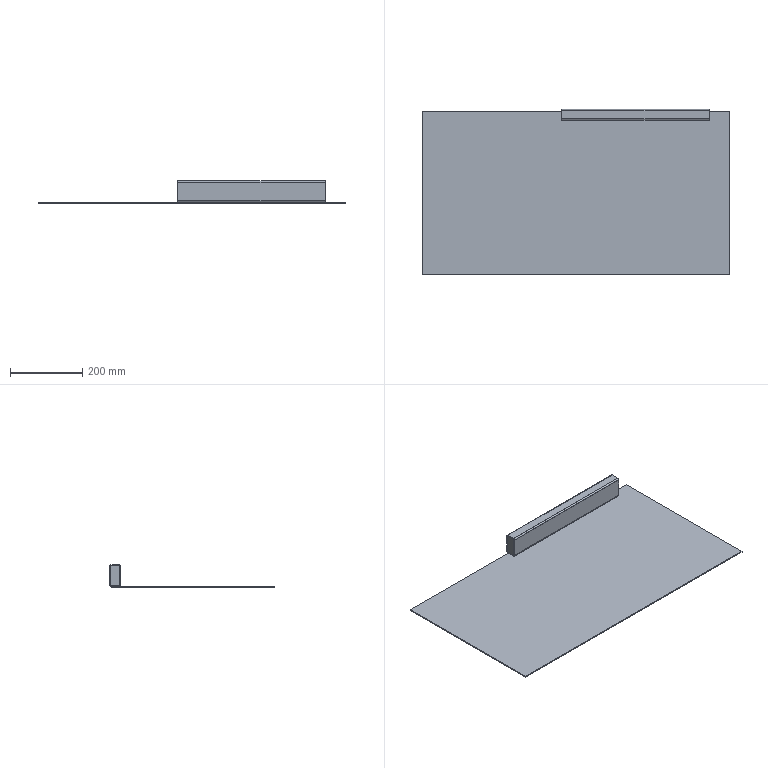Part | SolidWorks | features EndCap 1, Extrusion 1, WeldMemberFeat 1, WeldmentFeature 1 | 3 solids | 34 faces | box 850 x 458 x 63 mm | volume 1296033 mm3 | plane 22 | cylinder 12 | commonest cylinder face diameters 4 x8 8 x4
STEP:
#1=CARTESIAN_POINT('',(425.,-226.5,-1.5));
#2=VERTEX_POINT('',#1);
#3=CARTESIAN_POINT('',(425.,226.5,-1.5));
#4=VERTEX_POINT('',#3);
#5=CARTESIAN_POINT('',(425.,226.5,-1.5));
#6=DIRECTION('',(0.,1.,0.));
#7=VECTOR('',#6,1000.);
#8=LINE('',#5,#7);
#9=EDGE_CURVE('',#2,#4,#8,.T.);
#10=ORIENTED_EDGE('',*,*,#9,.T.);
#11=CARTESIAN_POINT('',(425.,226.5,1.5));
#12=VERTEX_POINT('',#11);
#13=CARTESIAN_POINT('',(425.,226.5,1.5));
#14=DIRECTION('',(0.,0.,-1.));
#15=VECTOR('',#14,1000.);
#16=LINE('',#13,#15);
#17=EDGE_CURVE('',#12,#4,#16,.T.);
#18=ORIENTED_EDGE('',*,*,#17,.F.);
#19=CARTESIAN_POINT('',(425.,-226.5,1.5));
#20=VERTEX_POINT('',#19);
#21=CARTESIAN_POINT('',(425.,226.5,1.5));
#22=DIRECTION('',(0.,1.,0.));
#23=VECTOR('',#22,1000.);
#24=LINE('',#21,#23);
#25=EDGE_CURVE('',#20,#12,#24,.T.);
#26=ORIENTED_EDGE('',*,*,#25,.F.);
#27=CARTESIAN_POINT('',(425.,-226.5,1.5));
#28=DIRECTION('',(0.,0.,-1.));
#29=VECTOR('',#28,1000.);
#30=LINE('',#27,#29);
#31=EDGE_CURVE('',#20,#2,#30,.T.);
#32=ORIENTED_EDGE('',*,*,#31,.T.);
#33=EDGE_LOOP('',(#10,#18,#26,#32));
#34=FACE_OUTER_BOUND('',#33,.T.);
#35=CARTESIAN_POINT('',(425.,226.5,1.5));
#36=DIRECTION('',(-1.,0.,0.));
#37=DIRECTION('',(0.,0.,1.));
#38=AXIS2_PLACEMENT_3D('',#35,#36,#37);
#39=PLANE('',#38);
#40=ADVANCED_FACE('',(#34),#39,.F.);
#41=CARTESIAN_POINT('',(-425.,226.5,-1.5));
#42=VERTEX_POINT('',#41);
#43=CARTESIAN_POINT('',(-425.,226.5,-1.5));
#44=DIRECTION('',(-1.,0.,0.));
#45=VECTOR('',#44,1000.);
#46=LINE('',#43,#45);
#47=EDGE_CURVE('',#4,#42,#46,.T.);
#48=ORIENTED_EDGE('',*,*,#47,.T.);
#49=CARTESIAN_POINT('',(-425.,226.5,1.5));
#50=VERTEX_POINT('',#49);
#51=CARTESIAN_POINT('',(-425.,226.5,1.5));
#52=DIRECTION('',(0.,0.,-1.));
#53=VECTOR('',#52,1000.);
#54=LINE('',#51,#53);
#55=EDGE_CURVE('',#50,#42,#54,.T.);
#56=ORIENTED_EDGE('',*,*,#55,.F.);
#57=CARTESIAN_POINT('',(-425.,226.5,1.5));
#58=DIRECTION('',(-1.,0.,0.));
#59=VECTOR('',#58,1000.);
#60=LINE('',#57,#59);
#61=EDGE_CURVE('',#12,#50,#60,.T.);
#62=ORIENTED_EDGE('',*,*,#61,.F.);
#63=ORIENTED_EDGE('',*,*,#17,.T.);
#64=EDGE_LOOP('',(#48,#56,#62,#63));
#65=FACE_OUTER_BOUND('',#64,.T.);
#66=CARTESIAN_POINT('',(-425.,226.5,1.5));
#67=DIRECTION('',(0.,-1.,0.));
#68=DIRECTION('',(0.,0.,-1.));
#69=AXIS2_PLACEMENT_3D('',#66,#67,#68);
#70=PLANE('',#69);
#71=ADVANCED_FACE('',(#65),#70,.F.);
#72=CARTESIAN_POINT('',(-425.,-226.5,-1.5));
#73=VERTEX_POINT('',#72);
#74=CARTESIAN_POINT('',(-425.,226.5,-1.5));
#75=DIRECTION('',(0.,-1.,0.));
#76=VECTOR('',#75,1000.);
#77=LINE('',#74,#76);
#78=EDGE_CURVE('',#42,#73,#77,.T.);
#79=ORIENTED_EDGE('',*,*,#78,.T.);
#80=CARTESIAN_POINT('',(-425.,-226.5,1.5));
#81=VERTEX_POINT('',#80);
#82=CARTESIAN_POINT('',(-425.,-226.5,1.5));
#83=DIRECTION('',(0.,0.,-1.));
#84=VECTOR('',#83,1000.);
#85=LINE('',#82,#84);
#86=EDGE_CURVE('',#81,#73,#85,.T.);
#87=ORIENTED_EDGE('',*,*,#86,.F.);
#88=CARTESIAN_POINT('',(-425.,226.5,1.5));
#89=DIRECTION('',(0.,-1.,0.));
#90=VECTOR('',#89,1000.);
#91=LINE('',#88,#90);
#92=EDGE_CURVE('',#50,#81,#91,.T.);
#93=ORIENTED_EDGE('',*,*,#92,.F.);
#94=ORIENTED_EDGE('',*,*,#55,.T.);
#95=EDGE_LOOP('',(#79,#87,#93,#94));
#96=FACE_OUTER_BOUND('',#95,.T.);
#97=CARTESIAN_POINT('',(-425.,226.5,1.5));
#98=DIRECTION('',(1.,0.,0.));
#99=DIRECTION('',(0.,0.,-1.));
#100=AXIS2_PLACEMENT_3D('',#97,#98,#99);
#101=PLANE('',#100);
#102=ADVANCED_FACE('',(#96),#101,.F.);
#103=CARTESIAN_POINT('',(-425.,-226.5,-1.5));
#104=DIRECTION('',(1.,0.,0.));
#105=VECTOR('',#104,1000.);
#106=LINE('',#103,#105);
#107=EDGE_CURVE('',#73,#2,#106,.T.);
#108=ORIENTED_EDGE('',*,*,#107,.T.);
#109=ORIENTED_EDGE('',*,*,#31,.F.);
#110=CARTESIAN_POINT('',(-425.,-226.5,1.5));
#111=DIRECTION('',(1.,0.,0.));
#112=VECTOR('',#111,1000.);
#113=LINE('',#110,#112);
#114=EDGE_CURVE('',#81,#20,#113,.T.);
#115=ORIENTED_EDGE('',*,*,#114,.F.);
#116=ORIENTED_EDGE('',*,*,#86,.T.);
#117=EDGE_LOOP('',(#108,#109,#115,#116));
#118=FACE_OUTER_BOUND('',#117,.T.);
#119=CARTESIAN_POINT('',(-425.,-226.5,1.5));
#120=DIRECTION('',(0.,1.,0.));
#121=DIRECTION('',(0.,0.,1.));
#122=AXIS2_PLACEMENT_3D('',#119,#120,#121);
#123=PLANE('',#122);
#124=ADVANCED_FACE('',(#118),#123,.F.);
#125=ORIENTED_EDGE('',*,*,#25,.T.);
#126=ORIENTED_EDGE('',*,*,#61,.T.);
#127=ORIENTED_EDGE('',*,*,#92,.T.);
#128=ORIENTED_EDGE('',*,*,#114,.T.);
#129=EDGE_LOOP('',(#125,#126,#127,#128));
#130=FACE_OUTER_BOUND('',#129,.T.);
#131=CARTESIAN_POINT('',(0.,0.,1.5));
#132=DIRECTION('',(0.,0.,1.));
#133=DIRECTION('',(1.,0.,0.));
#134=AXIS2_PLACEMENT_3D('',#131,#132,#133);
#135=PLANE('',#134);
#136=ADVANCED_FACE('',(#130),#135,.T.);
#137=ORIENTED_EDGE('',*,*,#9,.F.);
#138=ORIENTED_EDGE('',*,*,#107,.F.);
#139=ORIENTED_EDGE('',*,*,#78,.F.);
#140=ORIENTED_EDGE('',*,*,#47,.F.);
#141=EDGE_LOOP('',(#137,#138,#139,#140));
#142=FACE_OUTER_BOUND('',#141,.T.);
#143=CARTESIAN_POINT('',(0.,0.,-1.5));
#144=DIRECTION('',(0.,0.,1.));
#145=DIRECTION('',(1.,0.,0.));
#146=AXIS2_PLACEMENT_3D('',#143,#144,#145);
#147=PLANE('',#146);
#148=ADVANCED_FACE('',(#142),#147,.F.);
#149=CLOSED_SHELL('',(#40,#71,#102,#124,#136,#148));
#150=MANIFOLD_SOLID_BREP('',#149);
#151=CARTESIAN_POINT('',(370.,201.5,57.5));
#152=VERTEX_POINT('',#151);
#153=CARTESIAN_POINT('',(370.,205.5,61.5));
#154=VERTEX_POINT('',#153);
#155=CARTESIAN_POINT('',(370.,205.5,57.5));
#156=DIRECTION('',(-1.,0.,0.));
#157=DIRECTION('',(0.,-1.,0.));
#158=AXIS2_PLACEMENT_3D('',#155,#156,#157);
#159=CIRCLE('',#158,4.);
#160=EDGE_CURVE('',#152,#154,#159,.T.);
#161=ORIENTED_EDGE('',*,*,#160,.T.);
#162=CARTESIAN_POINT('',(-40.,205.5,61.5));
#163=VERTEX_POINT('',#162);
#164=CARTESIAN_POINT('',(-40.,205.5,61.5));
#165=DIRECTION('',(1.,0.,0.));
#166=VECTOR('',#165,1000.);
#167=LINE('',#164,#166);
#168=EDGE_CURVE('',#163,#154,#167,.T.);
#169=ORIENTED_EDGE('',*,*,#168,.F.);
#170=CARTESIAN_POINT('',(-40.,201.5,57.5));
#171=VERTEX_POINT('',#170);
#172=CARTESIAN_POINT('',(-40.,205.5,57.5));
#173=DIRECTION('',(-1.,0.,0.));
#174=DIRECTION('',(0.,-1.,0.));
#175=AXIS2_PLACEMENT_3D('',#172,#173,#174);
#176=CIRCLE('',#175,4.);
#177=EDGE_CURVE('',#171,#163,#176,.T.);
#178=ORIENTED_EDGE('',*,*,#177,.F.);
#179=CARTESIAN_POINT('',(-40.,201.5,57.5));
#180=DIRECTION('',(1.,0.,0.));
#181=VECTOR('',#180,1000.);
#182=LINE('',#179,#181);
#183=EDGE_CURVE('',#171,#152,#182,.T.);
#184=ORIENTED_EDGE('',*,*,#183,.T.);
#185=EDGE_LOOP('',(#161,#169,#178,#184));
#186=FACE_OUTER_BOUND('',#185,.T.);
#187=CARTESIAN_POINT('',(-40.,205.5,57.5));
#188=DIRECTION('',(1.,0.,0.));
#189=DIRECTION('',(0.,1.,0.));
#190=AXIS2_PLACEMENT_3D('',#187,#188,#189);
#191=CYLINDRICAL_SURFACE('',#190,4.);
#192=ADVANCED_FACE('',(#186),#191,.T.);
#193=CARTESIAN_POINT('',(370.,227.5,61.5));
#194=VERTEX_POINT('',#193);
#195=CARTESIAN_POINT('',(370.,205.5,61.5));
#196=DIRECTION('',(0.,1.,0.));
#197=VECTOR('',#196,1000.);
#198=LINE('',#195,#197);
#199=EDGE_CURVE('',#154,#194,#198,.T.);
#200=ORIENTED_EDGE('',*,*,#199,.T.);
#201=CARTESIAN_POINT('',(-40.,227.5,61.5));
#202=VERTEX_POINT('',#201);
#203=CARTESIAN_POINT('',(-40.,227.5,61.5));
#204=DIRECTION('',(1.,0.,0.));
#205=VECTOR('',#204,1000.);
#206=LINE('',#203,#205);
#207=EDGE_CURVE('',#202,#194,#206,.T.);
#208=ORIENTED_EDGE('',*,*,#207,.F.);
#209=CARTESIAN_POINT('',(-40.,205.5,61.5));
#210=DIRECTION('',(0.,1.,0.));
#211=VECTOR('',#210,1000.);
#212=LINE('',#209,#211);
#213=EDGE_CURVE('',#163,#202,#212,.T.);
#214=ORIENTED_EDGE('',*,*,#213,.F.);
#215=ORIENTED_EDGE('',*,*,#168,.T.);
#216=EDGE_LOOP('',(#200,#208,#214,#215));
#217=FACE_OUTER_BOUND('',#216,.T.);
#218=CARTESIAN_POINT('',(-40.,205.5,61.5));
#219=DIRECTION('',(0.,0.,-1.));
#220=DIRECTION('',(-1.,0.,0.));
#221=AXIS2_PLACEMENT_3D('',#218,#219,#220);
#222=PLANE('',#221);
#223=ADVANCED_FACE('',(#217),#222,.F.);
#224=CARTESIAN_POINT('',(370.,231.5,57.5));
#225=VERTEX_POINT('',#224);
#226=CARTESIAN_POINT('',(370.,227.5,57.5));
#227=DIRECTION('',(-1.,0.,0.));
#228=DIRECTION('',(0.,-1.,0.));
#229=AXIS2_PLACEMENT_3D('',#226,#227,#228);
#230=CIRCLE('',#229,4.);
#231=EDGE_CURVE('',#194,#225,#230,.T.);
#232=ORIENTED_EDGE('',*,*,#231,.T.);
#233=CARTESIAN_POINT('',(-40.,231.5,57.5));
#234=VERTEX_POINT('',#233);
#235=CARTESIAN_POINT('',(-40.,231.5,57.5));
#236=DIRECTION('',(1.,0.,0.));
#237=VECTOR('',#236,1000.);
#238=LINE('',#235,#237);
#239=EDGE_CURVE('',#234,#225,#238,.T.);
#240=ORIENTED_EDGE('',*,*,#239,.F.);
#241=CARTESIAN_POINT('',(-40.,227.5,57.5));
#242=DIRECTION('',(-1.,0.,0.));
#243=DIRECTION('',(0.,-1.,0.));
#244=AXIS2_PLACEMENT_3D('',#241,#242,#243);
#245=CIRCLE('',#244,4.);
#246=EDGE_CURVE('',#202,#234,#245,.T.);
#247=ORIENTED_EDGE('',*,*,#246,.F.);
#248=ORIENTED_EDGE('',*,*,#207,.T.);
#249=EDGE_LOOP('',(#232,#240,#247,#248));
#250=FACE_OUTER_BOUND('',#249,.T.);
#251=CARTESIAN_POINT('',(-40.,227.5,57.5));
#252=DIRECTION('',(1.,0.,0.));
#253=DIRECTION('',(0.,1.,0.));
#254=AXIS2_PLACEMENT_3D('',#251,#252,#253);
#255=CYLINDRICAL_SURFACE('',#254,4.);
#256=ADVANCED_FACE('',(#250),#255,.T.);
#257=CARTESIAN_POINT('',(370.,231.5,5.5));
#258=VERTEX_POINT('',#257);
#259=CARTESIAN_POINT('',(370.,231.5,5.5));
#260=DIRECTION('',(0.,0.,-1.));
#261=VECTOR('',#260,1000.);
#262=LINE('',#259,#261);
#263=EDGE_CURVE('',#225,#258,#262,.T.);
#264=ORIENTED_EDGE('',*,*,#263,.T.);
#265=CARTESIAN_POINT('',(-40.,231.5,5.5));
#266=VERTEX_POINT('',#265);
#267=CARTESIAN_POINT('',(-40.,231.5,5.5));
#268=DIRECTION('',(1.,0.,0.));
#269=VECTOR('',#268,1000.);
#270=LINE('',#267,#269);
#271=EDGE_CURVE('',#266,#258,#270,.T.);
#272=ORIENTED_EDGE('',*,*,#271,.F.);
#273=CARTESIAN_POINT('',(-40.,231.5,5.5));
#274=DIRECTION('',(0.,0.,-1.));
#275=VECTOR('',#274,1000.);
#276=LINE('',#273,#275);
#277=EDGE_CURVE('',#234,#266,#276,.T.);
#278=ORIENTED_EDGE('',*,*,#277,.F.);
#279=ORIENTED_EDGE('',*,*,#239,.T.);
#280=EDGE_LOOP('',(#264,#272,#278,#279));
#281=FACE_OUTER_BOUND('',#280,.T.);
#282=CARTESIAN_POINT('',(-40.,231.5,5.5));
#283=DIRECTION('',(0.,-1.,0.));
#284=DIRECTION('',(1.,0.,0.));
#285=AXIS2_PLACEMENT_3D('',#282,#283,#284);
#286=PLANE('',#285);
#287=ADVANCED_FACE('',(#281),#286,.F.);
#288=CARTESIAN_POINT('',(370.,227.5,1.5));
#289=VERTEX_POINT('',#288);
#290=CARTESIAN_POINT('',(370.,227.5,5.5));
#291=DIRECTION('',(-1.,0.,0.));
#292=DIRECTION('',(0.,-1.,0.));
#293=AXIS2_PLACEMENT_3D('',#290,#291,#292);
#294=CIRCLE('',#293,4.);
#295=EDGE_CURVE('',#258,#289,#294,.T.);
#296=ORIENTED_EDGE('',*,*,#295,.T.);
#297=CARTESIAN_POINT('',(-40.,227.5,1.5));
#298=VERTEX_POINT('',#297);
#299=CARTESIAN_POINT('',(-40.,227.5,1.5));
#300=DIRECTION('',(1.,0.,0.));
#301=VECTOR('',#300,1000.);
#302=LINE('',#299,#301);
#303=EDGE_CURVE('',#298,#289,#302,.T.);
#304=ORIENTED_EDGE('',*,*,#303,.F.);
#305=CARTESIAN_POINT('',(-40.,227.5,5.5));
#306=DIRECTION('',(-1.,0.,0.));
#307=DIRECTION('',(0.,-1.,0.));
#308=AXIS2_PLACEMENT_3D('',#305,#306,#307);
#309=CIRCLE('',#308,4.);
#310=EDGE_CURVE('',#266,#298,#309,.T.);
#311=ORIENTED_EDGE('',*,*,#310,.F.);
#312=ORIENTED_EDGE('',*,*,#271,.T.);
#313=EDGE_LOOP('',(#296,#304,#311,#312));
#314=FACE_OUTER_BOUND('',#313,.T.);
#315=CARTESIAN_POINT('',(-40.,227.5,5.5));
#316=DIRECTION('',(1.,0.,0.));
#317=DIRECTION('',(0.,1.,0.));
#318=AXIS2_PLACEMENT_3D('',#315,#316,#317);
#319=CYLINDRICAL_SURFACE('',#318,4.);
#320=ADVANCED_FACE('',(#314),#319,.T.);
#321=CARTESIAN_POINT('',(370.,205.5,1.5));
#322=VERTEX_POINT('',#321);
#323=CARTESIAN_POINT('',(370.,227.5,1.5));
#324=DIRECTION('',(0.,-1.,0.));
#325=VECTOR('',#324,1000.);
#326=LINE('',#323,#325);
#327=EDGE_CURVE('',#289,#322,#326,.T.);
#328=ORIENTED_EDGE('',*,*,#327,.T.);
#329=CARTESIAN_POINT('',(-40.,205.5,1.5));
#330=VERTEX_POINT('',#329);
#331=CARTESIAN_POINT('',(-40.,205.5,1.5));
#332=DIRECTION('',(1.,0.,0.));
#333=VECTOR('',#332,1000.);
#334=LINE('',#331,#333);
#335=EDGE_CURVE('',#330,#322,#334,.T.);
#336=ORIENTED_EDGE('',*,*,#335,.F.);
#337=CARTESIAN_POINT('',(-40.,227.5,1.5));
#338=DIRECTION('',(0.,-1.,0.));
#339=VECTOR('',#338,1000.);
#340=LINE('',#337,#339);
#341=EDGE_CURVE('',#298,#330,#340,.T.);
#342=ORIENTED_EDGE('',*,*,#341,.F.);
#343=ORIENTED_EDGE('',*,*,#303,.T.);
#344=EDGE_LOOP('',(#328,#336,#342,#343));
#345=FACE_OUTER_BOUND('',#344,.T.);
#346=CARTESIAN_POINT('',(-40.,227.5,1.5));
#347=DIRECTION('',(0.,0.,1.));
#348=DIRECTION('',(1.,0.,0.));
#349=AXIS2_PLACEMENT_3D('',#346,#347,#348);
#350=PLANE('',#349);
#351=ADVANCED_FACE('',(#345),#350,.F.);
#352=CARTESIAN_POINT('',(370.,201.5,5.5));
#353=VERTEX_POINT('',#352);
#354=CARTESIAN_POINT('',(370.,205.5,5.5));
#355=DIRECTION('',(-1.,0.,0.));
#356=DIRECTION('',(0.,-1.,0.));
#357=AXIS2_PLACEMENT_3D('',#354,#355,#356);
#358=CIRCLE('',#357,4.);
#359=EDGE_CURVE('',#322,#353,#358,.T.);
#360=ORIENTED_EDGE('',*,*,#359,.T.);
#361=CARTESIAN_POINT('',(-40.,201.5,5.5));
#362=VERTEX_POINT('',#361);
#363=CARTESIAN_POINT('',(-40.,201.5,5.5));
#364=DIRECTION('',(1.,0.,0.));
#365=VECTOR('',#364,1000.);
#366=LINE('',#363,#365);
#367=EDGE_CURVE('',#362,#353,#366,.T.);
#368=ORIENTED_EDGE('',*,*,#367,.F.);
#369=CARTESIAN_POINT('',(-40.,205.5,5.5));
#370=DIRECTION('',(-1.,0.,0.));
#371=DIRECTION('',(0.,-1.,0.));
#372=AXIS2_PLACEMENT_3D('',#369,#370,#371);
#373=CIRCLE('',#372,4.);
#374=EDGE_CURVE('',#330,#362,#373,.T.);
#375=ORIENTED_EDGE('',*,*,#374,.F.);
#376=ORIENTED_EDGE('',*,*,#335,.T.);
#377=EDGE_LOOP('',(#360,#368,#375,#376));
#378=FACE_OUTER_BOUND('',#377,.T.);
#379=CARTESIAN_POINT('',(-40.,205.5,5.5));
#380=DIRECTION('',(1.,0.,0.));
#381=DIRECTION('',(0.,1.,0.));
#382=AXIS2_PLACEMENT_3D('',#379,#380,#381);
#383=CYLINDRICAL_SURFACE('',#382,4.);
#384=ADVANCED_FACE('',(#378),#383,.T.);
#385=CARTESIAN_POINT('',(370.,227.5,59.5));
#386=VERTEX_POINT('',#385);
#387=CARTESIAN_POINT('',(370.,229.5,57.5));
#388=VERTEX_POINT('',#387);
#389=CARTESIAN_POINT('',(370.,227.5,57.5));
#390=DIRECTION('',(-1.,0.,0.));
#391=DIRECTION('',(0.,-1.,0.));
#392=AXIS2_PLACEMENT_3D('',#389,#390,#391);
#393=CIRCLE('',#392,2.);
#394=EDGE_CURVE('',#386,#388,#393,.T.);
#395=ORIENTED_EDGE('',*,*,#394,.F.);
#396=CARTESIAN_POINT('',(-40.,227.5,59.5));
#397=VERTEX_POINT('',#396);
#398=CARTESIAN_POINT('',(-40.,227.5,59.5));
#399=DIRECTION('',(1.,0.,0.));
#400=VECTOR('',#399,1000.);
#401=LINE('',#398,#400);
#402=EDGE_CURVE('',#397,#386,#401,.T.);
#403=ORIENTED_EDGE('',*,*,#402,.F.);
#404=CARTESIAN_POINT('',(-40.,229.5,57.5));
#405=VERTEX_POINT('',#404);
#406=CARTESIAN_POINT('',(-40.,227.5,57.5));
#407=DIRECTION('',(-1.,0.,0.));
#408=DIRECTION('',(0.,-1.,0.));
#409=AXIS2_PLACEMENT_3D('',#406,#407,#408);
#410=CIRCLE('',#409,2.);
#411=EDGE_CURVE('',#397,#405,#410,.T.);
#412=ORIENTED_EDGE('',*,*,#411,.T.);
#413=CARTESIAN_POINT('',(-40.,229.5,57.5));
#414=DIRECTION('',(1.,0.,0.));
#415=VECTOR('',#414,1000.);
#416=LINE('',#413,#415);
#417=EDGE_CURVE('',#405,#388,#416,.T.);
#418=ORIENTED_EDGE('',*,*,#417,.T.);
#419=EDGE_LOOP('',(#395,#403,#412,#418));
#420=FACE_OUTER_BOUND('',#419,.T.);
#421=CARTESIAN_POINT('',(-40.,227.5,57.5));
#422=DIRECTION('',(1.,0.,0.));
#423=DIRECTION('',(0.,1.,0.));
#424=AXIS2_PLACEMENT_3D('',#421,#422,#423);
#425=CYLINDRICAL_SURFACE('',#424,2.);
#426=ADVANCED_FACE('',(#420),#425,.F.);
#427=CARTESIAN_POINT('',(370.,205.5,59.5));
#428=VERTEX_POINT('',#427);
#429=CARTESIAN_POINT('',(370.,205.5,59.5));
#430=DIRECTION('',(0.,1.,0.));
#431=VECTOR('',#430,1000.);
#432=LINE('',#429,#431);
#433=EDGE_CURVE('',#428,#386,#432,.T.);
#434=ORIENTED_EDGE('',*,*,#433,.F.);
#435=CARTESIAN_POINT('',(-40.,205.5,59.5));
#436=VERTEX_POINT('',#435);
#437=CARTESIAN_POINT('',(-40.,205.5,59.5));
#438=DIRECTION('',(1.,0.,0.));
#439=VECTOR('',#438,1000.);
#440=LINE('',#437,#439);
#441=EDGE_CURVE('',#436,#428,#440,.T.);
#442=ORIENTED_EDGE('',*,*,#441,.F.);
#443=CARTESIAN_POINT('',(-40.,205.5,59.5));
#444=DIRECTION('',(0.,1.,0.));
#445=VECTOR('',#444,1000.);
#446=LINE('',#443,#445);
#447=EDGE_CURVE('',#436,#397,#446,.T.);
#448=ORIENTED_EDGE('',*,*,#447,.T.);
#449=ORIENTED_EDGE('',*,*,#402,.T.);
#450=EDGE_LOOP('',(#434,#442,#448,#449));
#451=FACE_OUTER_BOUND('',#450,.T.);
#452=CARTESIAN_POINT('',(-40.,205.5,59.5));
#453=DIRECTION('',(0.,0.,-1.));
#454=DIRECTION('',(-1.,0.,0.));
#455=AXIS2_PLACEMENT_3D('',#452,#453,#454);
#456=PLANE('',#455);
#457=ADVANCED_FACE('',(#451),#456,.T.);
#458=CARTESIAN_POINT('',(370.,203.5,57.5));
#459=VERTEX_POINT('',#458);
#460=CARTESIAN_POINT('',(370.,205.5,57.5));
#461=DIRECTION('',(-1.,0.,0.));
#462=DIRECTION('',(0.,-1.,0.));
#463=AXIS2_PLACEMENT_3D('',#460,#461,#462);
#464=CIRCLE('',#463,2.);
#465=EDGE_CURVE('',#459,#428,#464,.T.);
#466=ORIENTED_EDGE('',*,*,#465,.F.);
#467=CARTESIAN_POINT('',(-40.,203.5,57.5));
#468=VERTEX_POINT('',#467);
#469=CARTESIAN_POINT('',(-40.,203.5,57.5));
#470=DIRECTION('',(1.,0.,0.));
#471=VECTOR('',#470,1000.);
#472=LINE('',#469,#471);
#473=EDGE_CURVE('',#468,#459,#472,.T.);
#474=ORIENTED_EDGE('',*,*,#473,.F.);
#475=CARTESIAN_POINT('',(-40.,205.5,57.5));
#476=DIRECTION('',(-1.,0.,0.));
#477=DIRECTION('',(0.,-1.,0.));
#478=AXIS2_PLACEMENT_3D('',#475,#476,#477);
#479=CIRCLE('',#478,2.);
#480=EDGE_CURVE('',#468,#436,#479,.T.);
#481=ORIENTED_EDGE('',*,*,#480,.T.);
#482=ORIENTED_EDGE('',*,*,#441,.T.);
#483=EDGE_LOOP('',(#466,#474,#481,#482));
#484=FACE_OUTER_BOUND('',#483,.T.);
#485=CARTESIAN_POINT('',(-40.,205.5,57.5));
#486=DIRECTION('',(1.,0.,0.));
#487=DIRECTION('',(0.,1.,0.));
#488=AXIS2_PLACEMENT_3D('',#485,#486,#487);
#489=CYLINDRICAL_SURFACE('',#488,2.);
#490=ADVANCED_FACE('',(#484),#489,.F.);
#491=CARTESIAN_POINT('',(370.,203.5,5.5));
#492=VERTEX_POINT('',#491);
#493=CARTESIAN_POINT('',(370.,203.5,57.5));
#494=DIRECTION('',(0.,0.,1.));
#495=VECTOR('',#494,1000.);
#496=LINE('',#493,#495);
#497=EDGE_CURVE('',#492,#459,#496,.T.);
#498=ORIENTED_EDGE('',*,*,#497,.F.);
#499=CARTESIAN_POINT('',(-40.,203.5,5.5));
#500=VERTEX_POINT('',#499);
#501=CARTESIAN_POINT('',(-40.,203.5,5.5));
#502=DIRECTION('',(1.,0.,0.));
#503=VECTOR('',#502,1000.);
#504=LINE('',#501,#503);
#505=EDGE_CURVE('',#500,#492,#504,.T.);
#506=ORIENTED_EDGE('',*,*,#505,.F.);
#507=CARTESIAN_POINT('',(-40.,203.5,57.5));
#508=DIRECTION('',(0.,0.,1.));
#509=VECTOR('',#508,1000.);
#510=LINE('',#507,#509);
#511=EDGE_CURVE('',#500,#468,#510,.T.);
#512=ORIENTED_EDGE('',*,*,#511,.T.);
#513=ORIENTED_EDGE('',*,*,#473,.T.);
#514=EDGE_LOOP('',(#498,#506,#512,#513));
#515=FACE_OUTER_BOUND('',#514,.T.);
#516=CARTESIAN_POINT('',(-40.,203.5,57.5));
#517=DIRECTION('',(0.,1.,0.));
#518=DIRECTION('',(-1.,0.,0.));
#519=AXIS2_PLACEMENT_3D('',#516,#517,#518);
#520=PLANE('',#519);
#521=ADVANCED_FACE('',(#515),#520,.T.);
#522=CARTESIAN_POINT('',(370.,205.5,3.5));
#523=VERTEX_POINT('',#522);
#524=CARTESIAN_POINT('',(370.,205.5,5.5));
#525=DIRECTION('',(-1.,0.,0.));
#526=DIRECTION('',(0.,-1.,0.));
#527=AXIS2_PLACEMENT_3D('',#524,#525,#526);
#528=CIRCLE('',#527,2.);
#529=EDGE_CURVE('',#523,#492,#528,.T.);
#530=ORIENTED_EDGE('',*,*,#529,.F.);
#531=CARTESIAN_POINT('',(-40.,205.5,3.5));
#532=VERTEX_POINT('',#531);
#533=CARTESIAN_POINT('',(-40.,205.5,3.5));
#534=DIRECTION('',(1.,0.,0.));
#535=VECTOR('',#534,1000.);
#536=LINE('',#533,#535);
#537=EDGE_CURVE('',#532,#523,#536,.T.);
#538=ORIENTED_EDGE('',*,*,#537,.F.);
#539=CARTESIAN_POINT('',(-40.,205.5,5.5));
#540=DIRECTION('',(-1.,0.,0.));
#541=DIRECTION('',(0.,-1.,0.));
#542=AXIS2_PLACEMENT_3D('',#539,#540,#541);
#543=CIRCLE('',#542,2.);
#544=EDGE_CURVE('',#532,#500,#543,.T.);
#545=ORIENTED_EDGE('',*,*,#544,.T.);
#546=ORIENTED_EDGE('',*,*,#505,.T.);
#547=EDGE_LOOP('',(#530,#538,#545,#546));
#548=FACE_OUTER_BOUND('',#547,.T.);
#549=CARTESIAN_POINT('',(-40.,205.5,5.5));
#550=DIRECTION('',(1.,0.,0.));
#551=DIRECTION('',(0.,1.,0.));
#552=AXIS2_PLACEMENT_3D('',#549,#550,#551);
#553=CYLINDRICAL_SURFACE('',#552,2.);
#554=ADVANCED_FACE('',(#548),#553,.F.);
#555=CARTESIAN_POINT('',(370.,227.5,3.5));
#556=VERTEX_POINT('',#555);
#557=CARTESIAN_POINT('',(370.,227.5,3.5));
#558=DIRECTION('',(0.,-1.,0.));
#559=VECTOR('',#558,1000.);
#560=LINE('',#557,#559);
#561=EDGE_CURVE('',#556,#523,#560,.T.);
#562=ORIENTED_EDGE('',*,*,#561,.F.);
#563=CARTESIAN_POINT('',(-40.,227.5,3.5));
#564=VERTEX_POINT('',#563);
#565=CARTESIAN_POINT('',(-40.,227.5,3.5));
#566=DIRECTION('',(1.,0.,0.));
#567=VECTOR('',#566,1000.);
#568=LINE('',#565,#567);
#569=EDGE_CURVE('',#564,#556,#568,.T.);
#570=ORIENTED_EDGE('',*,*,#569,.F.);
#571=CARTESIAN_POINT('',(-40.,227.5,3.5));
#572=DIRECTION('',(0.,-1.,0.));
#573=VECTOR('',#572,1000.);
#574=LINE('',#571,#573);
#575=EDGE_CURVE('',#564,#532,#574,.T.);
#576=ORIENTED_EDGE('',*,*,#575,.T.);
#577=ORIENTED_EDGE('',*,*,#537,.T.);
#578=EDGE_LOOP('',(#562,#570,#576,#577));
#579=FACE_OUTER_BOUND('',#578,.T.);
#580=CARTESIAN_POINT('',(-40.,227.5,3.5));
#581=DIRECTION('',(0.,0.,1.));
#582=DIRECTION('',(1.,0.,0.));
#583=AXIS2_PLACEMENT_3D('',#580,#581,#582);
#584=PLANE('',#583);
#585=ADVANCED_FACE('',(#579),#584,.T.);
#586=CARTESIAN_POINT('',(370.,229.5,5.5));
#587=VERTEX_POINT('',#586);
#588=CARTESIAN_POINT('',(370.,227.5,5.5));
#589=DIRECTION('',(-1.,0.,0.));
#590=DIRECTION('',(0.,-1.,0.));
#591=AXIS2_PLACEMENT_3D('',#588,#589,#590);
#592=CIRCLE('',#591,2.);
#593=EDGE_CURVE('',#587,#556,#592,.T.);
#594=ORIENTED_EDGE('',*,*,#593,.F.);
#595=CARTESIAN_POINT('',(-40.,229.5,5.5));
#596=VERTEX_POINT('',#595);
#597=CARTESIAN_POINT('',(-40.,229.5,5.5));
#598=DIRECTION('',(1.,0.,0.));
#599=VECTOR('',#598,1000.);
#600=LINE('',#597,#599);
#601=EDGE_CURVE('',#596,#587,#600,.T.);
#602=ORIENTED_EDGE('',*,*,#601,.F.);
#603=CARTESIAN_POINT('',(-40.,227.5,5.5));
#604=DIRECTION('',(-1.,0.,0.));
#605=DIRECTION('',(0.,-1.,0.));
#606=AXIS2_PLACEMENT_3D('',#603,#604,#605);
#607=CIRCLE('',#606,2.);
#608=EDGE_CURVE('',#596,#564,#607,.T.);
#609=ORIENTED_EDGE('',*,*,#608,.T.);
#610=ORIENTED_EDGE('',*,*,#569,.T.);
#611=EDGE_LOOP('',(#594,#602,#609,#610));
#612=FACE_OUTER_BOUND('',#611,.T.);
#613=CARTESIAN_POINT('',(-40.,227.5,5.5));
#614=DIRECTION('',(1.,0.,0.));
#615=DIRECTION('',(0.,1.,0.));
#616=AXIS2_PLACEMENT_3D('',#613,#614,#615);
#617=CYLINDRICAL_SURFACE('',#616,2.);
#618=ADVANCED_FACE('',(#612),#617,.F.);
#619=CARTESIAN_POINT('',(370.,229.5,5.5));
#620=DIRECTION('',(0.,0.,-1.));
#621=VECTOR('',#620,1000.);
#622=LINE('',#619,#621);
#623=EDGE_CURVE('',#388,#587,#622,.T.);
#624=ORIENTED_EDGE('',*,*,#623,.F.);
#625=ORIENTED_EDGE('',*,*,#417,.F.);
#626=CARTESIAN_POINT('',(-40.,229.5,5.5));
#627=DIRECTION('',(0.,0.,-1.));
#628=VECTOR('',#627,1000.);
#629=LINE('',#626,#628);
#630=EDGE_CURVE('',#405,#596,#629,.T.);
#631=ORIENTED_EDGE('',*,*,#630,.T.);
#632=ORIENTED_EDGE('',*,*,#601,.T.);
#633=EDGE_LOOP('',(#624,#625,#631,#632));
#634=FACE_OUTER_BOUND('',#633,.T.);
#635=CARTESIAN_POINT('',(-40.,229.5,5.5));
#636=DIRECTION('',(0.,-1.,0.));
#637=DIRECTION('',(1.,0.,0.));
#638=AXIS2_PLACEMENT_3D('',#635,#636,#637);
#639=PLANE('',#638);
#640=ADVANCED_FACE('',(#634),#639,.T.);
#641=CARTESIAN_POINT('',(370.,201.5,57.5));
#642=DIRECTION('',(0.,0.,1.));
#643=VECTOR('',#642,1000.);
#644=LINE('',#641,#643);
#645=EDGE_CURVE('',#353,#152,#644,.T.);
#646=ORIENTED_EDGE('',*,*,#645,.T.);
#647=ORIENTED_EDGE('',*,*,#183,.F.);
#648=CARTESIAN_POINT('',(-40.,201.5,57.5));
#649=DIRECTION('',(0.,0.,1.));
#650=VECTOR('',#649,1000.);
#651=LINE('',#648,#650);
#652=EDGE_CURVE('',#362,#171,#651,.T.);
#653=ORIENTED_EDGE('',*,*,#652,.F.);
#654=ORIENTED_EDGE('',*,*,#367,.T.);
#655=EDGE_LOOP('',(#646,#647,#653,#654));
#656=FACE_OUTER_BOUND('',#655,.T.);
#657=CARTESIAN_POINT('',(-40.,201.5,57.5));
#658=DIRECTION('',(0.,1.,0.));
#659=DIRECTION('',(-1.,0.,0.));
#660=AXIS2_PLACEMENT_3D('',#657,#658,#659);
#661=PLANE('',#660);
#662=ADVANCED_FACE('',(#656),#661,.F.);
#663=ORIENTED_EDGE('',*,*,#411,.F.);
#664=ORIENTED_EDGE('',*,*,#447,.F.);
#665=ORIENTED_EDGE('',*,*,#480,.F.);
#666=ORIENTED_EDGE('',*,*,#511,.F.);
#667=ORIENTED_EDGE('',*,*,#544,.F.);
#668=ORIENTED_EDGE('',*,*,#575,.F.);
#669=ORIENTED_EDGE('',*,*,#608,.F.);
#670=ORIENTED_EDGE('',*,*,#630,.F.);
#671=EDGE_LOOP('',(#663,#664,#665,#666,#667,#668,#669,#670));
#672=FACE_BOUND('',#671,.T.);
#673=ORIENTED_EDGE('',*,*,#177,.T.);
#674=ORIENTED_EDGE('',*,*,#213,.T.);
#675=ORIENTED_EDGE('',*,*,#246,.T.);
#676=ORIENTED_EDGE('',*,*,#277,.T.);
#677=ORIENTED_EDGE('',*,*,#310,.T.);
#678=ORIENTED_EDGE('',*,*,#341,.T.);
#679=ORIENTED_EDGE('',*,*,#374,.T.);
#680=ORIENTED_EDGE('',*,*,#652,.T.);
#681=EDGE_LOOP('',(#673,#674,#675,#676,#677,#678,#679,#680));
#682=FACE_OUTER_BOUND('',#681,.T.);
#683=CARTESIAN_POINT('',(-40.,205.5,57.5));
#684=DIRECTION('',(-1.,0.,0.));
#685=DIRECTION('',(0.,-1.,0.));
#686=AXIS2_PLACEMENT_3D('',#683,#684,#685);
#687=PLANE('',#686);
#688=ADVANCED_FACE('',(#672,#682),#687,.T.);
#689=ORIENTED_EDGE('',*,*,#394,.T.);
#690=ORIENTED_EDGE('',*,*,#623,.T.);
#691=ORIENTED_EDGE('',*,*,#593,.T.);
#692=ORIENTED_EDGE('',*,*,#561,.T.);
#693=ORIENTED_EDGE('',*,*,#529,.T.);
#694=ORIENTED_EDGE('',*,*,#497,.T.);
#695=ORIENTED_EDGE('',*,*,#465,.T.);
#696=ORIENTED_EDGE('',*,*,#433,.T.);
#697=EDGE_LOOP('',(#689,#690,#691,#692,#693,#694,#695,#696));
#698=FACE_BOUND('',#697,.T.);
#699=ORIENTED_EDGE('',*,*,#160,.F.);
#700=ORIENTED_EDGE('',*,*,#645,.F.);
#701=ORIENTED_EDGE('',*,*,#359,.F.);
#702=ORIENTED_EDGE('',*,*,#327,.F.);
#703=ORIENTED_EDGE('',*,*,#295,.F.);
#704=ORIENTED_EDGE('',*,*,#263,.F.);
#705=ORIENTED_EDGE('',*,*,#231,.F.);
#706=ORIENTED_EDGE('',*,*,#199,.F.);
#707=EDGE_LOOP('',(#699,#700,#701,#702,#703,#704,#705,#706));
#708=FACE_OUTER_BOUND('',#707,.T.);
#709=CARTESIAN_POINT('',(370.,205.5,57.5));
#710=DIRECTION('',(-1.,0.,0.));
#711=DIRECTION('',(0.,-1.,0.));
#712=AXIS2_PLACEMENT_3D('',#709,#710,#711);
#713=PLANE('',#712);
#714=ADVANCED_FACE('',(#698,#708),#713,.F.);
#715=CLOSED_SHELL('',(#192,#223,#256,#287,#320,#351,#384,#426,#457,#490,#521,#554,#585,#618,#640,#662,#688,#714));
#716=MANIFOLD_SOLID_BREP('',#715);
#717=CARTESIAN_POINT('',(-40.,204.1,56.9));
#718=VERTEX_POINT('',#717);
#719=CARTESIAN_POINT('',(-40.,204.1,6.1));
#720=VERTEX_POINT('',#719);
#721=CARTESIAN_POINT('',(-40.,204.1,58.9));
#722=DIRECTION('',(0.,0.,-1.));
#723=VECTOR('',#722,1000.);
#724=LINE('',#721,#723);
#725=EDGE_CURVE('',#718,#720,#724,.T.);
#726=ORIENTED_EDGE('',*,*,#725,.T.);
#727=CARTESIAN_POINT('',(-37.,204.1,6.1));
#728=VERTEX_POINT('',#727);
#729=CARTESIAN_POINT('',(-37.,204.1,6.1));
#730=DIRECTION('',(-1.,0.,0.));
#731=VECTOR('',#730,1000.);
#732=LINE('',#729,#731);
#733=EDGE_CURVE('',#728,#720,#732,.T.);
#734=ORIENTED_EDGE('',*,*,#733,.F.);
#735=CARTESIAN_POINT('',(-37.,204.1,56.9));
#736=VERTEX_POINT('',#735);
#737=CARTESIAN_POINT('',(-37.,204.1,58.9));
#738=DIRECTION('',(0.,0.,-1.));
#739=VECTOR('',#738,1000.);
#740=LINE('',#737,#739);
#741=EDGE_CURVE('',#736,#728,#740,.T.);
#742=ORIENTED_EDGE('',*,*,#741,.F.);
#743=CARTESIAN_POINT('',(-37.,204.1,56.9));
#744=DIRECTION('',(-1.,0.,0.));
#745=VECTOR('',#744,1000.);
#746=LINE('',#743,#745);
#747=EDGE_CURVE('',#736,#718,#746,.T.);
#748=ORIENTED_EDGE('',*,*,#747,.T.);
#749=EDGE_LOOP('',(#726,#734,#742,#748));
#750=FACE_OUTER_BOUND('',#749,.T.);
#751=CARTESIAN_POINT('',(-37.,204.1,58.9));
#752=DIRECTION('',(0.,1.,0.));
#753=DIRECTION('',(-1.,0.,0.));
#754=AXIS2_PLACEMENT_3D('',#751,#752,#753);
#755=PLANE('',#754);
#756=ADVANCED_FACE('',(#750),#755,.F.);
#757=CARTESIAN_POINT('',(-40.,206.1,4.1));
#758=VERTEX_POINT('',#757);
#759=CARTESIAN_POINT('',(-40.,206.1,6.1));
#760=DIRECTION('',(1.,0.,0.));
#761=DIRECTION('',(0.,0.,1.));
#762=AXIS2_PLACEMENT_3D('',#759,#760,#761);
#763=CIRCLE('',#762,2.);
#764=EDGE_CURVE('',#720,#758,#763,.T.);
#765=ORIENTED_EDGE('',*,*,#764,.T.);
#766=CARTESIAN_POINT('',(-37.,206.1,4.1));
#767=VERTEX_POINT('',#766);
#768=CARTESIAN_POINT('',(-37.,206.1,4.1));
#769=DIRECTION('',(-1.,0.,0.));
#770=VECTOR('',#769,1000.);
#771=LINE('',#768,#770);
#772=EDGE_CURVE('',#767,#758,#771,.T.);
#773=ORIENTED_EDGE('',*,*,#772,.F.);
#774=CARTESIAN_POINT('',(-37.,206.1,6.1));
#775=DIRECTION('',(1.,0.,0.));
#776=DIRECTION('',(0.,0.,1.));
#777=AXIS2_PLACEMENT_3D('',#774,#775,#776);
#778=CIRCLE('',#777,2.);
#779=EDGE_CURVE('',#728,#767,#778,.T.);
#780=ORIENTED_EDGE('',*,*,#779,.F.);
#781=ORIENTED_EDGE('',*,*,#733,.T.);
#782=EDGE_LOOP('',(#765,#773,#780,#781));
#783=FACE_OUTER_BOUND('',#782,.T.);
#784=CARTESIAN_POINT('',(-37.,206.1,6.1));
#785=DIRECTION('',(-1.,0.,0.));
#786=DIRECTION('',(0.,-1.,0.));
#787=AXIS2_PLACEMENT_3D('',#784,#785,#786);
#788=CYLINDRICAL_SURFACE('',#787,2.);
#789=ADVANCED_FACE('',(#783),#788,.T.);
#790=CARTESIAN_POINT('',(-40.,226.9,4.1));
#791=VERTEX_POINT('',#790);
#792=CARTESIAN_POINT('',(-40.,204.1,4.1));
#793=DIRECTION('',(0.,1.,0.));
#794=VECTOR('',#793,1000.);
#795=LINE('',#792,#794);
#796=EDGE_CURVE('',#758,#791,#795,.T.);
#797=ORIENTED_EDGE('',*,*,#796,.T.);
#798=CARTESIAN_POINT('',(-37.,226.9,4.1));
#799=VERTEX_POINT('',#798);
#800=CARTESIAN_POINT('',(-37.,226.9,4.1));
#801=DIRECTION('',(-1.,0.,0.));
#802=VECTOR('',#801,1000.);
#803=LINE('',#800,#802);
#804=EDGE_CURVE('',#799,#791,#803,.T.);
#805=ORIENTED_EDGE('',*,*,#804,.F.);
#806=CARTESIAN_POINT('',(-37.,204.1,4.1));
#807=DIRECTION('',(0.,1.,0.));
#808=VECTOR('',#807,1000.);
#809=LINE('',#806,#808);
#810=EDGE_CURVE('',#767,#799,#809,.T.);
#811=ORIENTED_EDGE('',*,*,#810,.F.);
#812=ORIENTED_EDGE('',*,*,#772,.T.);
#813=EDGE_LOOP('',(#797,#805,#811,#812));
#814=FACE_OUTER_BOUND('',#813,.T.);
#815=CARTESIAN_POINT('',(-37.,204.1,4.1));
#816=DIRECTION('',(0.,0.,1.));
#817=DIRECTION('',(0.,-1.,0.));
#818=AXIS2_PLACEMENT_3D('',#815,#816,#817);
#819=PLANE('',#818);
#820=ADVANCED_FACE('',(#814),#819,.F.);
#821=CARTESIAN_POINT('',(-40.,228.9,6.1));
#822=VERTEX_POINT('',#821);
#823=CARTESIAN_POINT('',(-40.,226.9,6.1));
#824=DIRECTION('',(1.,0.,0.));
#825=DIRECTION('',(0.,0.,1.));
#826=AXIS2_PLACEMENT_3D('',#823,#824,#825);
#827=CIRCLE('',#826,2.);
#828=EDGE_CURVE('',#791,#822,#827,.T.);
#829=ORIENTED_EDGE('',*,*,#828,.T.);
#830=CARTESIAN_POINT('',(-37.,228.9,6.1));
#831=VERTEX_POINT('',#830);
#832=CARTESIAN_POINT('',(-37.,228.9,6.1));
#833=DIRECTION('',(-1.,0.,0.));
#834=VECTOR('',#833,1000.);
#835=LINE('',#832,#834);
#836=EDGE_CURVE('',#831,#822,#835,.T.);
#837=ORIENTED_EDGE('',*,*,#836,.F.);
#838=CARTESIAN_POINT('',(-37.,226.9,6.1));
#839=DIRECTION('',(1.,0.,0.));
#840=DIRECTION('',(0.,0.,1.));
#841=AXIS2_PLACEMENT_3D('',#838,#839,#840);
#842=CIRCLE('',#841,2.);
#843=EDGE_CURVE('',#799,#831,#842,.T.);
#844=ORIENTED_EDGE('',*,*,#843,.F.);
#845=ORIENTED_EDGE('',*,*,#804,.T.);
#846=EDGE_LOOP('',(#829,#837,#844,#845));
#847=FACE_OUTER_BOUND('',#846,.T.);
#848=CARTESIAN_POINT('',(-37.,226.9,6.1));
#849=DIRECTION('',(-1.,0.,0.));
#850=DIRECTION('',(0.,-1.,0.));
#851=AXIS2_PLACEMENT_3D('',#848,#849,#850);
#852=CYLINDRICAL_SURFACE('',#851,2.);
#853=ADVANCED_FACE('',(#847),#852,.T.);
#854=CARTESIAN_POINT('',(-40.,228.9,56.9));
#855=VERTEX_POINT('',#854);
#856=CARTESIAN_POINT('',(-40.,228.9,4.1));
#857=DIRECTION('',(0.,0.,1.));
#858=VECTOR('',#857,1000.);
#859=LINE('',#856,#858);
#860=EDGE_CURVE('',#822,#855,#859,.T.);
#861=ORIENTED_EDGE('',*,*,#860,.T.);
#862=CARTESIAN_POINT('',(-37.,228.9,56.9));
#863=VERTEX_POINT('',#862);
#864=CARTESIAN_POINT('',(-37.,228.9,56.9));
#865=DIRECTION('',(-1.,0.,0.));
#866=VECTOR('',#865,1000.);
#867=LINE('',#864,#866);
#868=EDGE_CURVE('',#863,#855,#867,.T.);
#869=ORIENTED_EDGE('',*,*,#868,.F.);
#870=CARTESIAN_POINT('',(-37.,228.9,4.1));
#871=DIRECTION('',(0.,0.,1.));
#872=VECTOR('',#871,1000.);
#873=LINE('',#870,#872);
#874=EDGE_CURVE('',#831,#863,#873,.T.);
#875=ORIENTED_EDGE('',*,*,#874,.F.);
#876=ORIENTED_EDGE('',*,*,#836,.T.);
#877=EDGE_LOOP('',(#861,#869,#875,#876));
#878=FACE_OUTER_BOUND('',#877,.T.);
#879=CARTESIAN_POINT('',(-37.,228.9,4.1));
#880=DIRECTION('',(0.,-1.,0.));
#881=DIRECTION('',(1.,0.,0.));
#882=AXIS2_PLACEMENT_3D('',#879,#880,#881);
#883=PLANE('',#882);
#884=ADVANCED_FACE('',(#878),#883,.F.);
#885=CARTESIAN_POINT('',(-40.,226.9,58.9));
#886=VERTEX_POINT('',#885);
#887=CARTESIAN_POINT('',(-40.,226.9,56.9));
#888=DIRECTION('',(1.,0.,0.));
#889=DIRECTION('',(0.,0.,1.));
#890=AXIS2_PLACEMENT_3D('',#887,#888,#889);
#891=CIRCLE('',#890,2.);
#892=EDGE_CURVE('',#855,#886,#891,.T.);
#893=ORIENTED_EDGE('',*,*,#892,.T.);
#894=CARTESIAN_POINT('',(-37.,226.9,58.9));
#895=VERTEX_POINT('',#894);
#896=CARTESIAN_POINT('',(-37.,226.9,58.9));
#897=DIRECTION('',(-1.,0.,0.));
#898=VECTOR('',#897,1000.);
#899=LINE('',#896,#898);
#900=EDGE_CURVE('',#895,#886,#899,.T.);
#901=ORIENTED_EDGE('',*,*,#900,.F.);
#902=CARTESIAN_POINT('',(-37.,226.9,56.9));
#903=DIRECTION('',(1.,0.,0.));
#904=DIRECTION('',(0.,0.,1.));
#905=AXIS2_PLACEMENT_3D('',#902,#903,#904);
#906=CIRCLE('',#905,2.);
#907=EDGE_CURVE('',#863,#895,#906,.T.);
#908=ORIENTED_EDGE('',*,*,#907,.F.);
#909=ORIENTED_EDGE('',*,*,#868,.T.);
#910=EDGE_LOOP('',(#893,#901,#908,#909));
#911=FACE_OUTER_BOUND('',#910,.T.);
#912=CARTESIAN_POINT('',(-37.,226.9,56.9));
#913=DIRECTION('',(-1.,0.,0.));
#914=DIRECTION('',(0.,-1.,0.));
#915=AXIS2_PLACEMENT_3D('',#912,#913,#914);
#916=CYLINDRICAL_SURFACE('',#915,2.);
#917=ADVANCED_FACE('',(#911),#916,.T.);
#918=CARTESIAN_POINT('',(-40.,206.1,58.9));
#919=VERTEX_POINT('',#918);
#920=CARTESIAN_POINT('',(-40.,228.9,58.9));
#921=DIRECTION('',(0.,-1.,0.));
#922=VECTOR('',#921,1000.);
#923=LINE('',#920,#922);
#924=EDGE_CURVE('',#886,#919,#923,.T.);
#925=ORIENTED_EDGE('',*,*,#924,.T.);
#926=CARTESIAN_POINT('',(-37.,206.1,58.9));
#927=VERTEX_POINT('',#926);
#928=CARTESIAN_POINT('',(-37.,206.1,58.9));
#929=DIRECTION('',(-1.,0.,0.));
#930=VECTOR('',#929,1000.);
#931=LINE('',#928,#930);
#932=EDGE_CURVE('',#927,#919,#931,.T.);
#933=ORIENTED_EDGE('',*,*,#932,.F.);
#934=CARTESIAN_POINT('',(-37.,228.9,58.9));
#935=DIRECTION('',(0.,-1.,0.));
#936=VECTOR('',#935,1000.);
#937=LINE('',#934,#936);
#938=EDGE_CURVE('',#895,#927,#937,.T.);
#939=ORIENTED_EDGE('',*,*,#938,.F.);
#940=ORIENTED_EDGE('',*,*,#900,.T.);
#941=EDGE_LOOP('',(#925,#933,#939,#940));
#942=FACE_OUTER_BOUND('',#941,.T.);
#943=CARTESIAN_POINT('',(-37.,228.9,58.9));
#944=DIRECTION('',(0.,0.,-1.));
#945=DIRECTION('',(0.,1.,0.));
#946=AXIS2_PLACEMENT_3D('',#943,#944,#945);
#947=PLANE('',#946);
#948=ADVANCED_FACE('',(#942),#947,.F.);
#949=CARTESIAN_POINT('',(-40.,206.1,56.9));
#950=DIRECTION('',(1.,0.,0.));
#951=DIRECTION('',(0.,0.,1.));
#952=AXIS2_PLACEMENT_3D('',#949,#950,#951);
#953=CIRCLE('',#952,2.);
#954=EDGE_CURVE('',#919,#718,#953,.T.);
#955=ORIENTED_EDGE('',*,*,#954,.T.);
#956=ORIENTED_EDGE('',*,*,#747,.F.);
#957=CARTESIAN_POINT('',(-37.,206.1,56.9));
#958=DIRECTION('',(1.,0.,0.));
#959=DIRECTION('',(0.,0.,1.));
#960=AXIS2_PLACEMENT_3D('',#957,#958,#959);
#961=CIRCLE('',#960,2.);
#962=EDGE_CURVE('',#927,#736,#961,.T.);
#963=ORIENTED_EDGE('',*,*,#962,.F.);
#964=ORIENTED_EDGE('',*,*,#932,.T.);
#965=EDGE_LOOP('',(#955,#956,#963,#964));
#966=FACE_OUTER_BOUND('',#965,.T.);
#967=CARTESIAN_POINT('',(-37.,206.1,56.9));
#968=DIRECTION('',(-1.,0.,0.));
#969=DIRECTION('',(0.,-1.,0.));
#970=AXIS2_PLACEMENT_3D('',#967,#968,#969);
#971=CYLINDRICAL_SURFACE('',#970,2.);
#972=ADVANCED_FACE('',(#966),#971,.T.);
#973=ORIENTED_EDGE('',*,*,#741,.T.);
#974=ORIENTED_EDGE('',*,*,#779,.T.);
#975=ORIENTED_EDGE('',*,*,#810,.T.);
#976=ORIENTED_EDGE('',*,*,#843,.T.);
#977=ORIENTED_EDGE('',*,*,#874,.T.);
#978=ORIENTED_EDGE('',*,*,#907,.T.);
#979=ORIENTED_EDGE('',*,*,#938,.T.);
#980=ORIENTED_EDGE('',*,*,#962,.T.);
#981=EDGE_LOOP('',(#973,#974,#975,#976,#977,#978,#979,#980));
#982=FACE_OUTER_BOUND('',#981,.T.);
#983=CARTESIAN_POINT('',(-37.,206.1,6.1));
#984=DIRECTION('',(-1.,0.,0.));
#985=DIRECTION('',(0.,0.,1.));
#986=AXIS2_PLACEMENT_3D('',#983,#984,#985);
#987=PLANE('',#986);
#988=ADVANCED_FACE('',(#982),#987,.F.);
#989=ORIENTED_EDGE('',*,*,#725,.F.);
#990=ORIENTED_EDGE('',*,*,#954,.F.);
#991=ORIENTED_EDGE('',*,*,#924,.F.);
#992=ORIENTED_EDGE('',*,*,#892,.F.);
#993=ORIENTED_EDGE('',*,*,#860,.F.);
#994=ORIENTED_EDGE('',*,*,#828,.F.);
#995=ORIENTED_EDGE('',*,*,#796,.F.);
#996=ORIENTED_EDGE('',*,*,#764,.F.);
#997=EDGE_LOOP('',(#989,#990,#991,#992,#993,#994,#995,#996));
#998=FACE_OUTER_BOUND('',#997,.T.);
#999=CARTESIAN_POINT('',(-40.,206.1,6.1));
#1000=DIRECTION('',(-1.,0.,0.));
#1001=DIRECTION('',(0.,0.,1.));
#1002=AXIS2_PLACEMENT_3D('',#999,#1000,#1001);
#1003=PLANE('',#1002);
#1004=ADVANCED_FACE('',(#998),#1003,.T.);
#1005=CLOSED_SHELL('',(#756,#789,#820,#853,#884,#917,#948,#972,#988,#1004));
#1006=MANIFOLD_SOLID_BREP('',#1005);
#1007=CARTESIAN_POINT('',(0.,0.,0.));
#1008=DIRECTION('',(0.,0.,1.));
#1009=DIRECTION('',(1.,0.,0.));
#1010=AXIS2_PLACEMENT_3D('',#1007,#1008,#1009);
#1011=(LENGTH_UNIT()NAMED_UNIT(*)SI_UNIT(.MILLI.,.METRE.));
#1012=UNCERTAINTY_MEASURE_WITH_UNIT(LENGTH_MEASURE(0.00001),#1011,'','');
#1013=(NAMED_UNIT(*)PLANE_ANGLE_UNIT()SI_UNIT($,.RADIAN.));
#1014=(NAMED_UNIT(*)SI_UNIT($,.STERADIAN.)SOLID_ANGLE_UNIT());
#1015=(GEOMETRIC_REPRESENTATION_CONTEXT(3)GLOBAL_UNCERTAINTY_ASSIGNED_CONTEXT((#1012))GLOBAL_UNIT_ASSIGNED_CONTEXT((#1011,#1013,#1014))REPRESENTATION_CONTEXT('',''));
#1016=ADVANCED_BREP_SHAPE_REPRESENTATION('',(#150,#716,#1006,#1010),#1015);